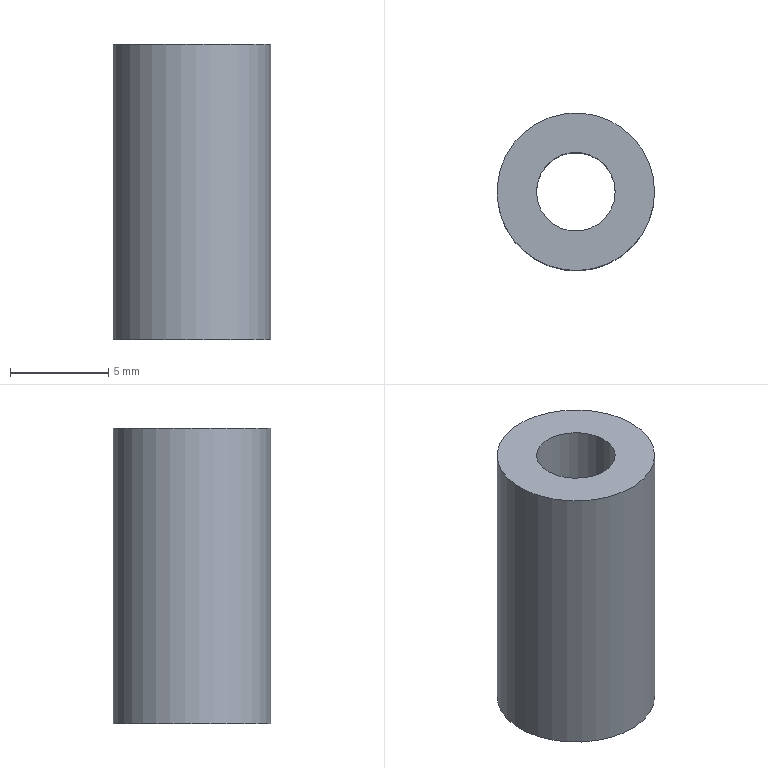Part | STEP file | gslz 2016.10.28-10_id2698_x_t | 1 solid | 4 faces | box 8 x 8 x 15 mm | volume 565.487 mm3 | cylinder 2 | plane 2 | commonest cylinder face diameters 4 x1 8 x1
STEP:
#1=CARTESIAN_POINT('',(0.,0.,0.));
#2=DIRECTION('',(0.,0.,1.));
#3=DIRECTION('',(1.,0.,0.));
#4=AXIS2_PLACEMENT_3D('',#1,#2,#3);
#5=CARTESIAN_POINT('',(-11.,40.,30.));
#6=VERTEX_POINT('',#5);
#7=CARTESIAN_POINT('',(-15.,40.,30.));
#8=DIRECTION('',(0.,0.,1.));
#9=DIRECTION('',(1.,0.,0.));
#10=AXIS2_PLACEMENT_3D('',#7,#8,#9);
#11=CIRCLE('',#10,4.);
#12=CARTESIAN_POINT('',(-15.,40.,58.));
#13=DIRECTION('',(0.,0.,-1.));
#14=DIRECTION('',(1.,0.,0.));
#15=AXIS2_PLACEMENT_3D('',#12,#13,#14);
#16=CYLINDRICAL_SURFACE('',#15,4.);
#17=CARTESIAN_POINT('',(6.283,28.));
#18=DIRECTION('',(-1.,0.));
#19=VECTOR('',#18,1.);
#20=LINE('',#17,#19);
#21=(GEOMETRIC_REPRESENTATION_CONTEXT(2)PARAMETRIC_REPRESENTATION_CONTEXT()REPRESENTATION_CONTEXT('',''));
#22=DEFINITIONAL_REPRESENTATION('',(#20),#21);
#23=PCURVE('',#16,#22);
#24=CARTESIAN_POINT('',(-15.,40.,30.));
#25=DIRECTION('',(0.,0.,1.));
#26=DIRECTION('',(-1.,0.,0.));
#27=AXIS2_PLACEMENT_3D('',#24,#25,#26);
#28=PLANE('',#27);
#29=CARTESIAN_POINT('',(0.,0.));
#30=DIRECTION('',(-1.,0.));
#31=AXIS2_PLACEMENT_2D('',#29,#30);
#32=CIRCLE('',#31,4.);
#33=(GEOMETRIC_REPRESENTATION_CONTEXT(2)PARAMETRIC_REPRESENTATION_CONTEXT()REPRESENTATION_CONTEXT('',''));
#34=DEFINITIONAL_REPRESENTATION('',(#32),#33);
#35=PCURVE('',#28,#34);
#36=SURFACE_CURVE('',#11,(#23,#35),.PCURVE_S1.);
#37=EDGE_CURVE('',#6,#6,#36,.T.);
#38=ORIENTED_EDGE('',*,*,#37,.F.);
#39=CARTESIAN_POINT('',(-11.,40.,15.));
#40=VERTEX_POINT('',#39);
#41=CARTESIAN_POINT('',(-11.,40.,30.));
#42=CARTESIAN_POINT('',(-11.,40.,15.));
#43=B_SPLINE_CURVE_WITH_KNOTS('',1,(#41,#42),.UNSPECIFIED.,.F.,.F.,(2,2),(28.,43.),.PIECEWISE_BEZIER_KNOTS.);
#44=CARTESIAN_POINT('',(6.283,0.));
#45=DIRECTION('',(0.,1.));
#46=VECTOR('',#45,1.);
#47=LINE('',#44,#46);
#48=(GEOMETRIC_REPRESENTATION_CONTEXT(2)PARAMETRIC_REPRESENTATION_CONTEXT()REPRESENTATION_CONTEXT('',''));
#49=DEFINITIONAL_REPRESENTATION('',(#47),#48);
#50=PCURVE('',#16,#49);
#51=CARTESIAN_POINT('',(0.,0.));
#52=DIRECTION('',(0.,1.));
#53=VECTOR('',#52,1.);
#54=LINE('',#51,#53);
#55=(GEOMETRIC_REPRESENTATION_CONTEXT(2)PARAMETRIC_REPRESENTATION_CONTEXT()REPRESENTATION_CONTEXT('',''));
#56=DEFINITIONAL_REPRESENTATION('',(#54),#55);
#57=PCURVE('',#16,#56);
#58=SEAM_CURVE('',#43,(#50,#57),.PCURVE_S1.);
#59=EDGE_CURVE('',#6,#40,#58,.T.);
#60=ORIENTED_EDGE('',*,*,#59,.T.);
#61=CARTESIAN_POINT('',(-15.,40.,15.));
#62=DIRECTION('',(0.,0.,1.));
#63=DIRECTION('',(1.,0.,0.));
#64=AXIS2_PLACEMENT_3D('',#61,#62,#63);
#65=CIRCLE('',#64,4.);
#66=CARTESIAN_POINT('',(6.283,43.));
#67=DIRECTION('',(-1.,0.));
#68=VECTOR('',#67,1.);
#69=LINE('',#66,#68);
#70=(GEOMETRIC_REPRESENTATION_CONTEXT(2)PARAMETRIC_REPRESENTATION_CONTEXT()REPRESENTATION_CONTEXT('',''));
#71=DEFINITIONAL_REPRESENTATION('',(#69),#70);
#72=PCURVE('',#16,#71);
#73=CARTESIAN_POINT('',(-15.,40.,15.));
#74=DIRECTION('',(0.,0.,1.));
#75=DIRECTION('',(-1.,0.,0.));
#76=AXIS2_PLACEMENT_3D('',#73,#74,#75);
#77=PLANE('',#76);
#78=CARTESIAN_POINT('',(0.,0.));
#79=DIRECTION('',(-1.,0.));
#80=AXIS2_PLACEMENT_2D('',#78,#79);
#81=CIRCLE('',#80,4.);
#82=(GEOMETRIC_REPRESENTATION_CONTEXT(2)PARAMETRIC_REPRESENTATION_CONTEXT()REPRESENTATION_CONTEXT('',''));
#83=DEFINITIONAL_REPRESENTATION('',(#81),#82);
#84=PCURVE('',#77,#83);
#85=SURFACE_CURVE('',#65,(#72,#84),.PCURVE_S1.);
#86=EDGE_CURVE('',#40,#40,#85,.T.);
#87=ORIENTED_EDGE('',*,*,#86,.T.);
#88=ORIENTED_EDGE('',*,*,#59,.F.);
#89=EDGE_LOOP('',(#38,#60,#87,#88));
#90=FACE_BOUND('',#89,.T.);
#91=ADVANCED_FACE('',(#90),#16,.T.);
#92=CARTESIAN_POINT('',(-13.,40.,30.));
#93=VERTEX_POINT('',#92);
#94=CARTESIAN_POINT('',(-15.,40.,30.));
#95=DIRECTION('',(0.,0.,1.));
#96=DIRECTION('',(1.,0.,0.));
#97=AXIS2_PLACEMENT_3D('',#94,#95,#96);
#98=CIRCLE('',#97,2.);
#99=CARTESIAN_POINT('',(0.,0.));
#100=DIRECTION('',(-1.,0.));
#101=AXIS2_PLACEMENT_2D('',#99,#100);
#102=CIRCLE('',#101,2.);
#103=(GEOMETRIC_REPRESENTATION_CONTEXT(2)PARAMETRIC_REPRESENTATION_CONTEXT()REPRESENTATION_CONTEXT('',''));
#104=DEFINITIONAL_REPRESENTATION('',(#102),#103);
#105=PCURVE('',#28,#104);
#106=CARTESIAN_POINT('',(-15.,40.,-2.));
#107=DIRECTION('',(0.,0.,1.));
#108=DIRECTION('',(-1.,0.,0.));
#109=AXIS2_PLACEMENT_3D('',#106,#107,#108);
#110=CYLINDRICAL_SURFACE('',#109,2.);
#111=CARTESIAN_POINT('',(3.142,32.));
#112=DIRECTION('',(1.,0.));
#113=VECTOR('',#112,1.);
#114=LINE('',#111,#113);
#115=(GEOMETRIC_REPRESENTATION_CONTEXT(2)PARAMETRIC_REPRESENTATION_CONTEXT()REPRESENTATION_CONTEXT('',''));
#116=DEFINITIONAL_REPRESENTATION('',(#114),#115);
#117=PCURVE('',#110,#116);
#118=SURFACE_CURVE('',#98,(#105,#117),.PCURVE_S1.);
#119=EDGE_CURVE('',#93,#93,#118,.T.);
#120=ORIENTED_EDGE('',*,*,#119,.F.);
#121=EDGE_LOOP('',(#120));
#122=FACE_BOUND('',#121,.T.);
#123=ORIENTED_EDGE('',*,*,#37,.T.);
#124=EDGE_LOOP('',(#123));
#125=FACE_BOUND('',#124,.T.);
#126=ADVANCED_FACE('',(#122,#125),#28,.T.);
#127=CARTESIAN_POINT('',(-13.,40.,15.));
#128=VERTEX_POINT('',#127);
#129=CARTESIAN_POINT('',(-15.,40.,15.));
#130=DIRECTION('',(0.,0.,1.));
#131=DIRECTION('',(1.,0.,0.));
#132=AXIS2_PLACEMENT_3D('',#129,#130,#131);
#133=CIRCLE('',#132,2.);
#134=CARTESIAN_POINT('',(0.,0.));
#135=DIRECTION('',(-1.,0.));
#136=AXIS2_PLACEMENT_2D('',#134,#135);
#137=CIRCLE('',#136,2.);
#138=(GEOMETRIC_REPRESENTATION_CONTEXT(2)PARAMETRIC_REPRESENTATION_CONTEXT()REPRESENTATION_CONTEXT('',''));
#139=DEFINITIONAL_REPRESENTATION('',(#137),#138);
#140=PCURVE('',#77,#139);
#141=CARTESIAN_POINT('',(3.142,17.));
#142=DIRECTION('',(1.,0.));
#143=VECTOR('',#142,1.);
#144=LINE('',#141,#143);
#145=(GEOMETRIC_REPRESENTATION_CONTEXT(2)PARAMETRIC_REPRESENTATION_CONTEXT()REPRESENTATION_CONTEXT('',''));
#146=DEFINITIONAL_REPRESENTATION('',(#144),#145);
#147=PCURVE('',#110,#146);
#148=SURFACE_CURVE('',#133,(#140,#147),.PCURVE_S1.);
#149=EDGE_CURVE('',#128,#128,#148,.T.);
#150=ORIENTED_EDGE('',*,*,#149,.T.);
#151=EDGE_LOOP('',(#150));
#152=FACE_BOUND('',#151,.T.);
#153=ORIENTED_EDGE('',*,*,#86,.F.);
#154=EDGE_LOOP('',(#153));
#155=FACE_BOUND('',#154,.T.);
#156=ADVANCED_FACE('',(#152,#155),#77,.F.);
#157=ORIENTED_EDGE('',*,*,#119,.F.);
#158=CARTESIAN_POINT('',(-13.,40.,15.));
#159=CARTESIAN_POINT('',(-13.,40.,30.));
#160=B_SPLINE_CURVE_WITH_KNOTS('',1,(#158,#159),.UNSPECIFIED.,.F.,.F.,(2,2),(17.,32.),.PIECEWISE_BEZIER_KNOTS.);
#161=CARTESIAN_POINT('',(3.142,0.));
#162=DIRECTION('',(0.,1.));
#163=VECTOR('',#162,1.);
#164=LINE('',#161,#163);
#165=(GEOMETRIC_REPRESENTATION_CONTEXT(2)PARAMETRIC_REPRESENTATION_CONTEXT()REPRESENTATION_CONTEXT('',''));
#166=DEFINITIONAL_REPRESENTATION('',(#164),#165);
#167=PCURVE('',#110,#166);
#168=CARTESIAN_POINT('',(9.425,0.));
#169=DIRECTION('',(0.,1.));
#170=VECTOR('',#169,1.);
#171=LINE('',#168,#170);
#172=(GEOMETRIC_REPRESENTATION_CONTEXT(2)PARAMETRIC_REPRESENTATION_CONTEXT()REPRESENTATION_CONTEXT('',''));
#173=DEFINITIONAL_REPRESENTATION('',(#171),#172);
#174=PCURVE('',#110,#173);
#175=SEAM_CURVE('',#160,(#167,#174),.PCURVE_S1.);
#176=EDGE_CURVE('',#128,#93,#175,.T.);
#177=ORIENTED_EDGE('',*,*,#176,.F.);
#178=ORIENTED_EDGE('',*,*,#149,.T.);
#179=ORIENTED_EDGE('',*,*,#176,.T.);
#180=EDGE_LOOP('',(#157,#177,#178,#179));
#181=FACE_BOUND('',#180,.F.);
#182=ADVANCED_FACE('',(#181),#110,.F.);
#183=CLOSED_SHELL('',(#91,#126,#156,#182));
#184=MANIFOLD_SOLID_BREP('',#183);
#185=(LENGTH_UNIT()NAMED_UNIT(*)SI_UNIT(.MILLI.,.METRE.));
#186=UNCERTAINTY_MEASURE_WITH_UNIT(LENGTH_MEASURE(0.00001),#185,'','');
#187=(NAMED_UNIT(*)PLANE_ANGLE_UNIT()SI_UNIT($,.RADIAN.));
#188=(NAMED_UNIT(*)SI_UNIT($,.STERADIAN.)SOLID_ANGLE_UNIT());
#189=(GEOMETRIC_REPRESENTATION_CONTEXT(3)GLOBAL_UNCERTAINTY_ASSIGNED_CONTEXT((#186))GLOBAL_UNIT_ASSIGNED_CONTEXT((#185,#187,#188))REPRESENTATION_CONTEXT('',''));
#190=ADVANCED_BREP_SHAPE_REPRESENTATION('',(#4,#184),#189);